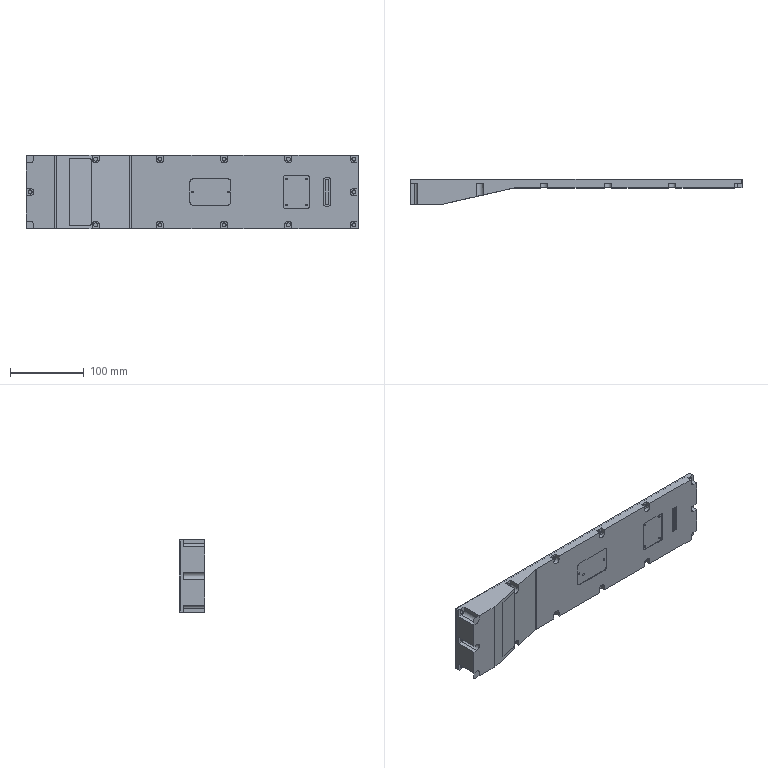NC program | Mastercam | posted with a generic post | part box 450 x 35 x 100 mm
Lines 24995 to 25762 of 140701:
(20 FEM |TOOL - 20|DIA. OFF. - 20|LEN. - 20|TOOL DIA. - 20.)
N556 T20 M6
N558 G0 G54 G90 X-118.202 Y-6.075 C0. B0. S7000 M3
N560 G43 H20 Z50.
N562 Z1.055
N564 G2 X-116.202 Y-4.075 Z1. I2. F4000.
N566 G3 X-97.202 Y14.925 Z.5 J19.
N568 X-116.202 Y33.925 Z0. I-19.
N570 X-135.202 Y14.925 Z-.5 J-19.
N572 X-116.202 Y-4.075 Z-1. I19.
N574 G1 X-91.853
N576 X-63.511
N578 G2 X-59.795 Y0. I43.131 J-35.6
N580 X-63.511 Y4.075 I39.415 J39.675
N582 G1 X-122.39
N584 Y-4.075
N586 X-116.202
N588 G2 X-114.191 Y-5.683 J-2.062
N590 G1 X-112.027 Y-15.257
N592 G3 X-110.015 Y-16.865 I2.012 J.455
N594 G1 X-91.853
N596 X-56.995
N598 G2 X-49.546 Y-7.894 I79.55 J-58.48
N600 X-41.146 Y-1.835 I29.252 J-31.701
N602 G1 X-37.436 Y0.
N604 X-41.146 Y1.835
N606 G2 X-49.546 Y7.894 I20.852 J37.76
N608 X-56.995 Y16.865 I72.101 J67.451
N610 G1 X-135.18
N612 Y-16.865
N614 X-110.015
N616 G3 X-108.015 Y-14.865 Z-.945 J2.
N618 G0 Z50.
N620 X42.897 Y-2.91
N622 Z1.
N624 G3 X51.894 Y-5.175 Z.843 I8.997 J16.735
N626 X68.629 Y4.827 Z.5 J19.
N628 X70.895 Y13.825 Z.343 I-16.735 J8.998
N630 X60.892 Y30.559 Z0. I-19.001
N632 X51.894 Y32.825 Z-.157 I-8.998 J-16.734
N634 X35.16 Y22.822 Z-.5 J-19.
N636 X32.895 Y13.825 Z-.657 I16.734 J-8.997
N638 X42.897 Y-2.91 Z-1. I18.999
N640 G2 X43.5 Y-3.234 I-391.044 J-727.301
N642 X49.572 Y0. I23.249 J-36.334
N644 X43.5 Y3.234 I17.177 J39.568
N646 X37.436 Y0. I-391.647 J726.977
N648 X42.897 Y-2.91 I-385.583 J-730.211
N650 G3 X43.844 Y-3.148 Z-.983 I.947 J1.762
N652 X45.605 Y-2.095 Z-.945 J2.
N654 G0 Z50.
N656 X129.904 Y-2.873
N658 Z1.
N660 G3 X139.687 Y-5.585 Z.828 I9.783 J16.288
N662 X155.975 Y3.632 Z.5 J19.
N664 X158.687 Y13.415 Z.328 I-16.288 J9.783
N666 X149.469 Y29.703 Z0. I-19.
N668 X139.687 Y32.415 Z-.172 I-9.782 J-16.288
N670 X123.399 Y23.197 Z-.5 J-19.
N672 X120.687 Y13.415 Z-.672 I16.288 J-9.782
N674 X129.904 Y-2.873 Z-1. I19.
N676 G2 X130.501 Y-3.237 I-27.641 J-46.024
N678 X136.397 Y-.078 I23.255 J-36.326
N680 G1 X136.575 Y0.
N682 X136.397 Y.078
N684 G2 X130.501 Y3.237 I17.359 J39.485
N686 X124.428 Y0. I-28.238 J45.66
N688 X129.904 Y-2.873 I-22.165 J-48.897
N690 X130.904 Y-4.641 I-1.062 J-1.768
N692 X130.837 Y-5.167 I-2.062
N694 G1 X128.644 Y-13.481
N696 G3 X128.576 Y-14.007 I1.995 J-.526
N698 X129.288 Y-15.566 I2.063
N700 G1 X130.501 Y-16.616
N702 G2 X135.006 Y-12.831 I23.174 J-23.004
N704 G1 X135.087 Y-12.774
N706 G2 X140.615 Y-9.672 I18.669 J-26.789
N708 G1 X140.702 Y-9.634
N710 G2 X146.548 Y-7.698 I13.141 J-29.891
N712 G1 X146.639 Y-7.677
N714 G2 X153.208 Y-6.86 I7.296 J-31.827
N716 G1 X153.401 Y-6.855
N718 X193.897 Y-6.847
N720 G2 X202.347 Y-7.916 I-1.055 J-42.291
N722 G1 Y7.916
N724 G2 X194.995 Y6.866 I-9.346 J39.174
N726 G1 X154.128 Y6.847
N728 X153.208 Y6.86
N730 G2 X146.639 Y7.677 I.727 J32.644
N732 G1 X146.548 Y7.698
N734 G2 X140.702 Y9.634 I7.295 J31.827
N736 G1 X140.615 Y9.672
N738 G2 X135.087 Y12.774 I13.141 J29.891
N740 G1 X135.006 Y12.831
N742 G2 X130.501 Y16.616 I18.669 J26.789
N744 G1 X126.823 Y13.429
N746 G2 X121.297 Y10.091 I-19.566 J26.142
N748 G1 X121.211 Y10.05
N750 G2 X109.473 Y6.942 I-14.658 J31.635
N752 G1 X109.381 Y6.935
N754 X67.041 Y6.847
N756 X66.081 Y6.861
N758 X60.698 Y7.454
N760 G2 X54.022 Y9.497 I6.163 J32.066
N762 G1 X53.91 Y9.545
N764 G2 X47.444 Y13.233 I12.839 J30.023
N766 G1 X43.499 Y16.616
N768 G2 X35.971 Y10.952 I-44.52 J51.336
N770 X25.649 Y7.333 I-16.878 J31.613
N772 G1 X20.337 Y6.85
N774 G2 X.051 Y6.761 I-20.286 J2311.595
N776 X-20.508 Y6.853 J2311.684
N778 X-30.199 Y8.456 I1.227 J37.504
N780 G1 X-30.263 Y8.477
N782 G2 X-35.971 Y10.952 I10.077 J31.059
N784 G1 X-36.079 Y11.012
N786 G2 X-42.437 Y15.598 I15.785 J28.583
N788 G1 X-42.523 Y15.677
N790 G2 X-47.502 Y21.493 I22.143 J23.998
N792 G1 X-47.568 Y21.591
N794 G2 X-50.642 Y27.347 I27.123 J18.181
N796 G1 X-145.662
N798 Y-27.347
N800 X-50.642
N802 G2 X-47.568 Y-21.591 I30.197 J-12.425
N804 G1 X-47.502 Y-21.493
N806 G2 X-42.523 Y-15.677 I27.122 J-18.182
N808 G1 X-42.437 Y-15.598
N810 G2 X-36.079 Y-11.012 I22.143 J-23.997
N812 G1 X-35.971 Y-10.952
N814 G2 X-30.263 Y-8.477 I15.785 J-28.584
N816 G1 X-30.199 Y-8.456
N818 G2 X-20.508 Y-6.853 I10.918 J-35.901
N820 X.051 Y-6.762 I20.559 J-2311.592
N822 X20.337 Y-6.85 J-2311.683
N824 G1 X25.649 Y-7.333
N826 G2 X35.971 Y-10.952 I-6.556 J-35.232
N828 X43.499 Y-16.616 I-36.992 J-57.
N830 G1 X47.444 Y-13.233
N832 G2 X53.91 Y-9.545 I19.305 J-26.335
N834 G1 X54.022 Y-9.497
N836 G2 X60.698 Y-7.454 I12.839 J-30.023
N838 G1 X60.788 Y-7.437
N840 G2 X67.041 Y-6.847 I6.861 J-39.333
N842 G1 X109.381 Y-6.935
N844 G2 X121.211 Y-10.05 I-2.812 J-34.699
N846 G1 X121.297 Y-10.091
N848 G2 X126.823 Y-13.429 I-14.04 J-29.48
N850 G1 X129.288 Y-15.566
N852 G2 X129.999 Y-17.124 I-1.351 J-1.558
N854 X129.767 Y-18.076 I-2.062
N856 G1 X124.991 Y-27.255
N858 G3 X124.758 Y-28.207 I1.83 J-.952
N860 X125.048 Y-29.262 I2.063
N862 G2 X128. Y-39.493 I-18.064 J-10.752
N864 G1 X133.001
N866 G2 X145.59 Y-20.752 I21.022 J-.523
N868 X153.478 Y-19.002 I8.921 J-21.56
N870 G1 X153.672 Y-18.998
N872 X193.897 Y-18.993
N874 X193.982
N876 G2 X214.493 Y-35.389 J-21.027
N878 G1 Y35.389
N880 G2 X194.768 Y19.011 I-20.505 J4.628
N882 G1 X194.587 Y19.005
N884 X153.672 Y18.998
N886 X149.261 Y19.537
N888 G2 X133.001 Y39.493 I4.758 J20.478
N890 G1 X128.
N892 G2 X112.383 Y19.696 I-21.016 J.521
N894 X106.99 Y18.993 I-13.4 J81.701
N896 G1 X66.495 Y19.
N898 G2 X54.539 Y23.091 I.65 J21.417
N900 X45.999 Y39.493 I12.534 J16.951
N902 G1 X41.
N904 G2 X39.774 Y32.921 I-49.58 J5.846
N906 G1 X39.731 Y32.803
N908 G2 X37.479 Y28.354 I-19.286 J6.969
N910 G1 X37.414 Y28.256
N912 G2 X34.287 Y24.604 I-17.034 J11.419
N914 G1 X34.201 Y24.524
N916 G2 X26.515 Y20.03 I-15.057 J16.929
N918 X20.337 Y18.997 I-7.888 J28.2
N920 X-.041 Y18.899 I-20.378 J2122.333
N922 X-20.166 Y18.995 J2122.431
N924 X-26.515 Y20.03 I1.337 J28.195
N926 X-34.287 Y24.604 I7.334 J21.352
N928 X-37.414 Y28.256 I13.907 J15.071
N930 G1 X-37.479 Y28.354
N932 G2 X-39.731 Y32.803 I17.034 J11.418
N934 X-41. Y39.493 I45.456 J12.083
N936 G1 X-157.808
N938 Y-39.493
N940 X-41.
N942 G2 X-39.774 Y-32.921 I49.58 J-5.846
N944 G1 X-39.731 Y-32.803
N946 G2 X-37.479 Y-28.354 I19.286 J-6.969
N948 G1 X-37.414 Y-28.256
N950 G2 X-34.287 Y-24.604 I17.034 J-11.419
N952 G1 X-34.201 Y-24.524
N954 G2 X-26.515 Y-20.03 I15.057 J-16.929
N956 X-20.337 Y-18.997 I7.888 J-28.2
N958 X.004 Y-18.899 I20.341 J-2118.094
N960 X19.878 Y-18.993 J-2118.192
N962 X26.515 Y-20.03 I-.812 J-26.956
N964 X34.201 Y-24.524 I-7.371 J-21.423
N966 G1 X34.287 Y-24.604
N968 G2 X37.414 Y-28.256 I-13.907 J-15.071
N970 G1 X37.479 Y-28.354
N972 G2 X39.731 Y-32.803 I-17.034 J-11.418
N974 X41. Y-39.493 I-45.456 J-12.083
N976 G1 X45.999
N978 G2 X51.434 Y-25.897 I21.203 J-.591
N980 X67.041 Y-18.993 I15.623 J-14.225
N982 G1 X106.99
N984 G2 X112.383 Y-19.696 I-8.007 J-82.404
N986 X125.048 Y-29.262 I-5.399 J-20.318
N988 X125.338 Y-30.316 I-1.772 J-1.054
N990 X124.805 Y-31.701 I-2.062
N992 G1 X118.034 Y-39.175
N994 G3 X117.5 Y-40.559 I1.528 J-1.385
N996 G1 X117.499 Y-50.
N998 X143.501
N1000 G2 X143.5 Y-49.884 I9.999 J.116
N1002 G1 X143.505 Y-39.753
N1004 X143.509 Y-39.626
N1006 G2 X143.82 Y-37.443 I9.995 J-.311
N1008 G1 X143.851 Y-37.322
N1010 G2 X144.5 Y-35.531 I9.684 J-2.493
N1012 G1 X144.527 Y-35.473
N1014 G2 X145.171 Y-34.319 I9.036 J-4.284
N1016 G1 X145.208 Y-34.262
N1018 G2 X146.3 Y-32.865 I8.392 J-5.438
N1020 G1 X146.375 Y-32.785
N1022 G2 X147.957 Y-31.416 I7.3 J-6.835
N1024 G1 X148.039 Y-31.359
N1026 G2 X149.732 Y-30.409 I5.717 J-8.204
N1028 G1 X149.818 Y-30.371
N1030 G2 X151.609 Y-29.778 I4.025 J-9.154
N1032 G1 X151.7 Y-29.757
N1034 G2 X153.712 Y-29.507 I2.235 J-9.747
N1036 G1 X153.905 Y-29.502
N1038 X193.897 Y-29.5
N1040 X194.414 Y-29.512
N1042 G2 X196.337 Y-29.765 I-.336 J-9.994
N1044 G1 X196.406 Y-29.781
N1046 G2 X197.7 Y-30.175 I-2.258 J-9.741
N1048 G1 X197.76 Y-30.197
N1050 G2 X199.353 Y-30.971 I-3.553 J-9.348
N1052 G1 X199.45 Y-31.029
N1054 G2 X201.184 Y-32.346 I-5.146 J-8.574
N1056 G1 X201.26 Y-32.418
N1058 G2 X202.596 Y-33.975 I-6.88 J-7.257
N1060 G1 X202.654 Y-34.058
N1062 G2 X203.635 Y-35.832 I-8.217 J-5.7
N1064 G1 X203.675 Y-35.926
N1066 G2 X204.291 Y-37.927 I-9.198 J-3.926
N1068 G1 X204.311 Y-38.033
N1070 G2 X204.497 Y-39.8 I-9.813 J-1.924
N1072 G1 X204.499 Y-39.917
N1074 Y-50.
N1076 X223.648
N1078 X223.993 Y-49.994
N1080 X224.033 Y-49.965
N1082 X224.98 Y-49.016
N1084 X224.995 Y-48.986
N1086 X225. Y-48.71
N1088 Y48.71
N1090 X224.995 Y48.986
N1092 X224.98 Y49.016
N1094 X224.033 Y49.965
N1096 X223.971 Y49.996
N1098 X204.499 Y50.
N1100 X204.5 Y40.074
N1102 X204.497 Y39.8
N1104 G2 X204.311 Y38.033 I-9.999 J.157
N1106 G1 X204.291 Y37.927
N1108 G2 X203.675 Y35.926 I-9.814 J1.925
N1110 G1 X203.635 Y35.832
N1112 G2 X202.654 Y34.058 I-9.198 J3.926
N1114 G1 X202.596 Y33.975
N1116 G2 X201.26 Y32.418 I-8.216 J5.7
N1118 G1 X201.184 Y32.346
N1120 G2 X199.45 Y31.029 I-6.88 J7.257
N1122 G1 X199.353 Y30.971
N1124 G2 X197.76 Y30.197 I-5.146 J8.574
N1126 G1 X197.7 Y30.175
N1128 G2 X196.406 Y29.781 I-3.552 J9.347
N1130 G1 X196.337 Y29.765
N1132 G2 X194.414 Y29.512 I-2.259 J9.741
N1134 G1 X193.897 Y29.5
N1136 X154.128
N1138 X153.712 Y29.507
N1140 G2 X151.7 Y29.757 I.223 J9.997
N1142 G1 X151.609 Y29.778
N1144 G2 X149.818 Y30.371 I2.234 J9.747
N1146 G1 X149.732 Y30.409
N1148 G2 X148.039 Y31.359 I4.024 J9.154
N1150 G1 X147.957 Y31.416
N1152 G2 X146.375 Y32.785 I5.718 J8.204
N1154 G1 X146.3 Y32.865
N1156 G2 X145.208 Y34.262 I7.3 J6.835
N1158 G1 X145.171 Y34.319
N1160 G2 X144.527 Y35.473 I8.392 J5.438
N1162 G1 X144.5 Y35.531
N1164 G2 X143.851 Y37.322 I9.035 J4.284
N1166 G1 X143.82 Y37.443
N1168 G2 X143.509 Y39.626 I9.684 J2.494
N1170 G1 X143.505 Y39.753
N1172 X143.501 Y50.
N1174 X117.499
N1176 X117.5 Y40.041
N1178 X117.458 Y39.11
N1180 G2 X117.074 Y37.042 I-9.97 J.783
N1182 G1 X117.053 Y36.973
N1184 G2 X116.533 Y35.602 I-9.585 J2.85
N1186 G1 X116.502 Y35.535
N1188 G2 X115.768 Y34.226 I-9.066 J4.221
N1190 G1 X115.726 Y34.162
N1192 G2 X114.752 Y32.92 I-8.332 J5.53
N1194 G1 X114.697 Y32.86
N1196 G2 X113.331 Y31.627 I-7.358 J6.773
N1198 G1 X113.249 Y31.565
N1200 G2 X111.557 Y30.543 I-5.992 J8.006
N1202 G1 X111.471 Y30.502
N1204 G2 X109.712 Y29.858 I-4.3 J9.028
N1206 G1 X109.623 Y29.835
N1208 G2 X107.814 Y29.534 I-2.541 J9.672
N1210 G1 X106.99 Y29.5
N1212 X67.041
N1214 X66.685 Y29.506
N1216 G2 X65.063 Y29.682 I.266 J9.996
N1218 G1 X64.974 Y29.699
N1220 G2 X62.929 Y30.325 I1.887 J9.821
N1222 G1 X62.817 Y30.373
N1224 G2 X60.837 Y31.503 I3.932 J9.195
N1226 G1 X60.751 Y31.565
N1228 G2 X59.237 Y32.933 I5.912 J8.065
N1230 G1 X59.171 Y33.006
N1232 G2 X58.019 Y34.565 I7.427 J6.697
N1234 G1 X57.97 Y34.647
N1236 G2 X57.146 Y36.381 I8.578 J5.138
N1238 G1 X57.113 Y36.472
N1240 G2 X56.627 Y38.39 I9.403 J3.404
N1242 G1 X56.612 Y38.49
N1244 G2 X56.501 Y39.95 I9.889 J1.486
N1246 G1 X56.5 Y40.166
N1248 X56.501 Y50.
N1250 X30.499
N1252 X30.5 Y40.036
N1254 X30.453 Y39.059
N1256 G2 X29.893 Y36.492 I-9.965 J.831
N1258 G1 X29.85 Y36.374
N1260 G2 X28.752 Y34.204 I-9.405 J3.398
N1262 G1 X28.686 Y34.107
N1264 G2 X27.161 Y32.325 I-8.306 J5.568
N1266 G1 X27.075 Y32.246
N1268 G2 X25.128 Y30.842 I-6.781 J7.349
N1270 G1 X25.02 Y30.782
N1272 G2 X23.272 Y30.024 I-4.834 J8.754
N1274 G1 X23.208 Y30.003
N1276 G2 X21.837 Y29.663 I-3.086 J9.512
N1278 G1 X21.764 Y29.651
N1280 G2 X20.19 Y29.503 I-1.715 J9.851
N1282 G1 X19.878 Y29.5
N1284 X-20.018 Y29.501
N1286 X-20.19 Y29.503
N1288 G2 X-21.764 Y29.651 I.141 J9.999
N1290 G1 X-21.837 Y29.663
N1292 G2 X-23.208 Y30.003 I1.715 J9.852
N1294 G1 X-23.272 Y30.024
N1296 G2 X-25.02 Y30.782 I3.086 J9.512
N1298 G1 X-25.128 Y30.842
N1300 G2 X-27.075 Y32.246 I4.834 J8.753
N1302 G1 X-27.161 Y32.325
N1304 G2 X-28.686 Y34.107 I6.781 J7.35
N1306 G1 X-28.752 Y34.204
N1308 G2 X-29.85 Y36.374 I8.307 J5.568
N1310 G1 X-29.893 Y36.492
N1312 G2 X-30.453 Y39.059 I9.405 J3.398
N1314 G1 X-30.5 Y40.036
N1316 X-30.499 Y50.
N1318 X-168.315
N1320 Y-50.
N1322 X-30.499
N1324 X-30.5 Y-40.036
N1326 X-30.453 Y-39.059
N1328 G2 X-29.893 Y-36.492 I9.965 J-.831
N1330 G1 X-29.85 Y-36.374
N1332 G2 X-28.752 Y-34.204 I9.405 J-3.398
N1334 G1 X-28.686 Y-34.107
N1336 G2 X-27.161 Y-32.325 I8.306 J-5.568
N1338 G1 X-27.075 Y-32.246
N1340 G2 X-25.128 Y-30.842 I6.781 J-7.349
N1342 G1 X-25.02 Y-30.782
N1344 G2 X-23.272 Y-30.024 I4.834 J-8.754
N1346 G1 X-23.208 Y-30.003
N1348 G2 X-21.837 Y-29.663 I3.086 J-9.512
N1350 G1 X-21.764 Y-29.651
N1352 G2 X-20.19 Y-29.503 I1.715 J-9.851
N1354 G1 X-19.878 Y-29.5
N1356 X20.018 Y-29.501
N1358 X20.19 Y-29.503
N1360 G2 X21.764 Y-29.651 I-.141 J-9.999
N1362 G1 X21.837 Y-29.663
N1364 G2 X23.208 Y-30.003 I-1.715 J-9.852
N1366 G1 X23.272 Y-30.024
N1368 G2 X25.02 Y-30.782 I-3.086 J-9.512
N1370 G1 X25.128 Y-30.842
N1372 G2 X27.075 Y-32.246 I-4.834 J-8.753
N1374 G1 X27.161 Y-32.325
N1376 G2 X28.686 Y-34.107 I-6.781 J-7.35
N1378 G1 X28.752 Y-34.204
N1380 G2 X29.85 Y-36.374 I-8.307 J-5.568
N1382 G1 X29.893 Y-36.492
N1384 G2 X30.453 Y-39.059 I-9.405 J-3.398
N1386 G1 X30.5 Y-40.036
N1388 X30.499 Y-50.
N1390 X56.501
N1392 Y-39.976
N1394 G2 X56.612 Y-38.49 I10.
N1396 G1 X56.627 Y-38.39
N1398 G2 X57.113 Y-36.472 I9.889 J-1.486
N1400 G1 X57.146 Y-36.381
N1402 G2 X57.97 Y-34.647 I9.402 J-3.404
N1404 G1 X58.019 Y-34.565
N1406 G2 X59.171 Y-33.006 I8.579 J-5.138
N1408 G1 X59.237 Y-32.933
N1410 G2 X60.751 Y-31.565 I7.426 J-6.697
N1412 G1 X60.837 Y-31.503
N1414 G2 X62.817 Y-30.373 I5.912 J-8.065
N1416 G1 X62.929 Y-30.325
N1418 G2 X64.974 Y-29.699 I3.932 J-9.195
N1420 G1 X65.063 Y-29.682
N1422 G2 X66.685 Y-29.506 I1.888 J-9.82
N1424 G1 X67.041 Y-29.5
N1426 X106.99
N1428 X107.814 Y-29.534
N1430 G2 X109.623 Y-29.835 I-.732 J-9.973
N1432 G1 X109.712 Y-29.858
N1434 G2 X111.471 Y-30.502 I-2.541 J-9.672
N1436 G1 X111.557 Y-30.543
N1438 G2 X113.249 Y-31.565 I-4.3 J-9.028
N1440 G1 X113.331 Y-31.627
N1442 G2 X114.697 Y-32.86 I-5.992 J-8.006
N1444 G1 X114.752 Y-32.92
N1446 G2 X115.726 Y-34.162 I-7.358 J-6.772
N1448 G1 X115.768 Y-34.226
N1450 G2 X116.502 Y-35.535 I-8.332 J-5.53
N1452 G1 X116.533 Y-35.602
N1454 G2 X117.053 Y-36.973 I-9.065 J-4.221
N1456 G1 X117.074 Y-37.042
N1458 G2 X117.458 Y-39.11 I-9.586 J-2.851
N1460 G1 X117.469 Y-39.258
N1462 G2 X117.5 Y-40.041 I-9.969 J-.783
N1464 G1 Y-40.559
N1466 Y-40.56
N1468 G3 X119.562 Y-42.622 I2.062
N1470 X121.427 Y-41.442 J2.062
N1472 G1 X145.254 Y8.886
N1474 G3 X147.082 Y17.017 Z-1.079 I-17.172 J8.131
N1476 X130.973 Y35.795 Z-1.333 I-19.
N1478 X128.082 Y36.016 Z-1.36 I-2.891 J-18.778
N1480 X109.083 Y17.017 Z-1.642 J-18.999
N1482 X109.259 Y14.429 Z-1.667 I18.999
N1484 X128.082 Y-1.983 Z-1.924 I18.823 J2.588
N1486 X135.933 Y-.285 Z-2. J19.
N1488 G2 X136.397 Y-.078 I17.823 J-39.278
N1490 G1 X136.575 Y0.
N1492 X136.397 Y.078
N1494 G2 X130.501 Y3.237 I17.359 J39.485
N1496 X124.428 Y0. I-28.238 J45.66
N1498 X130.501 Y-3.237 I-22.165 J-48.897
N1500 X135.933 Y-.285 I23.255 J-36.326
N1502 G3 X137.106 Y1.536 Z-1.96 I-.827 J1.821
N1504 X136.928 Y2.362 Z-1.945 I-2.
N1506 G0 Z50.
N1508 X44.092 Y2.862
N1510 Z0.
N1512 G3 X34.112 Y5.694 Z-.176 I-9.98 J-16.168
N1514 X17.944 Y-3.327 Z-.5 J-19.
N1516 X15.112 Y-13.306 Z-.676 I16.168 J-9.979
N1518 X24.133 Y-29.474 Z-1. I19.
N1520 X34.112 Y-32.306 Z-1.176 I9.979 J16.168
N1522 X50.28 Y-23.286 Z-1.5 J19.
N1524 X53.112 Y-13.306 Z-1.676 I-16.168 J9.98
N1526 X44.092 Y2.862 Z-2. I-19.
N1528 G2 X43.5 Y3.234 I22.657 J36.706
N1530 X37.436 Y0. I-391.647 J726.977
N1532 X43.5 Y-3.234 I-385.583 J-730.211
N1534 X49.572 Y0. I23.249 J-36.334
N1536 X44.092 Y2.862 I17.177 J39.568
N1538 G3 X43.042 Y3.16 Z-1.981 I-1.05 J-1.702
N1540 X41.34 Y2.21 Z-1.945 J-2.
N1542 G0 Z50.
N1544 X-64.181 Y4.075
N1546 Z0.
N1548 G3 X-83.181 Y-14.925 Z-.5 J-19.
N1550 X-64.181 Y-33.925 Z-1. I19.
N1552 X-45.181 Y-14.925 Z-1.5 J19.
N1554 X-64.181 Y4.075 Z-2. I-19.
N1556 G1 X-117.97
N1558 Y-4.075
N1560 X-89.643
N1562 X-63.511
N1564 G2 X-59.795 Y0. I43.131 J-35.6
N1566 X-63.511 Y4.075 I39.415 J39.675
N1568 G1 X-64.181
N1570 G2 X-66.193 Y5.683 J2.062
N1572 G1 X-68.357 Y15.257
N1574 G3 X-70.369 Y16.865 I-2.012 J-.455
N1576 G1 X-130.761
N1578 Y-16.865
N1580 X-89.643
N1582 X-56.995
N1584 G2 X-49.546 Y-7.894 I79.55 J-58.48
N1586 X-41.146 Y-1.835 I29.252 J-31.701
N1588 G1 X-37.436 Y0.
N1590 X-41.146 Y1.835
N1592 G2 X-49.546 Y7.894 I20.852 J37.76
N1594 X-56.995 Y16.865 I72.101 J67.451
N1596 G1 X-70.369
N1598 G2 X-72.346 Y18.341 J2.062
N1600 G1 X-74.579 Y25.871
N1602 G3 X-76.556 Y27.347 I-1.977 J-.586
N1604 G1 X-141.243
N1606 Y-27.347
N1608 X-50.642
N1610 G2 X-47.568 Y-21.591 I30.197 J-12.425
N1612 G1 X-47.502 Y-21.493
N1614 G2 X-42.523 Y-15.677 I27.122 J-18.182
N1616 G1 X-42.437 Y-15.598
N1618 G2 X-36.079 Y-11.012 I22.143 J-23.997
N1620 G1 X-35.971 Y-10.952
N1622 G2 X-30.263 Y-8.477 I15.785 J-28.584
N1624 G1 X-30.199 Y-8.456
N1626 G2 X-20.508 Y-6.853 I10.918 J-35.901
N1628 X.051 Y-6.762 I20.559 J-2311.592
N1630 X20.337 Y-6.85 J-2311.683
N1632 G1 X25.649 Y-7.333
N1634 G2 X35.971 Y-10.952 I-6.556 J-35.232
N1636 X43.499 Y-16.616 I-36.992 J-57.
N1638 G1 X47.444 Y-13.233
N1640 G2 X53.91 Y-9.545 I19.305 J-26.335
N1642 G1 X54.022 Y-9.497
N1644 G2 X60.698 Y-7.454 I12.839 J-30.023
N1646 G1 X60.788 Y-7.437
N1648 G2 X67.041 Y-6.847 I6.861 J-39.333
N1650 G1 X109.381 Y-6.935
N1652 G2 X121.211 Y-10.05 I-2.812 J-34.699
N1654 G1 X121.297 Y-10.091
N1656 G2 X126.823 Y-13.429 I-14.04 J-29.48
N1658 G1 X130.501 Y-16.616
N1660 G2 X135.006 Y-12.831 I23.174 J-23.004
N1662 G1 X135.087 Y-12.774
N1664 G2 X140.615 Y-9.672 I18.669 J-26.789
N1666 G1 X140.702 Y-9.634
N1668 G2 X146.548 Y-7.698 I13.141 J-29.891
N1670 G1 X146.639 Y-7.677
N1672 G2 X153.208 Y-6.86 I7.296 J-31.827
N1674 G1 X153.401 Y-6.855
N1676 X193.897 Y-6.847
N1678 G2 X202.347 Y-7.916 I-1.055 J-42.291
N1680 G1 Y7.916
N1682 G2 X194.995 Y6.866 I-9.346 J39.174
N1684 G1 X154.128 Y6.847
N1686 X153.208 Y6.86
N1688 G2 X146.639 Y7.677 I.727 J32.644
N1690 G1 X146.548 Y7.698
N1692 G2 X140.702 Y9.634 I7.295 J31.827
N1694 G1 X140.615 Y9.672
N1696 G2 X135.087 Y12.774 I13.141 J29.891
N1698 G1 X135.006 Y12.831
N1700 G2 X130.501 Y16.616 I18.669 J26.789
N1702 G1 X126.823 Y13.429
N1704 G2 X121.297 Y10.091 I-19.566 J26.142
N1706 G1 X121.211 Y10.05
N1708 G2 X109.473 Y6.942 I-14.658 J31.635
N1710 G1 X109.381 Y6.935
N1712 X67.041 Y6.847
N1714 X66.081 Y6.861
N1716 X60.698 Y7.454
N1718 G2 X54.022 Y9.497 I6.163 J32.066
N1720 G1 X53.91 Y9.545
N1722 G2 X47.444 Y13.233 I12.839 J30.023
N1724 G1 X43.499 Y16.616
N1726 G2 X35.971 Y10.952 I-44.52 J51.336
N1728 X25.649 Y7.333 I-16.878 J31.613
N1730 G1 X20.337 Y6.85
N1732 G2 X.051 Y6.761 I-20.286 J2311.595
N1734 X-20.508 Y6.853 J2311.684
N1736 X-30.199 Y8.456 I1.227 J37.504
N1738 G1 X-30.263 Y8.477
N1740 G2 X-35.971 Y10.952 I10.077 J31.059
N1742 G1 X-36.079 Y11.012
N1744 G2 X-42.437 Y15.598 I15.785 J28.583
N1746 G1 X-42.523 Y15.677
N1748 G2 X-47.502 Y21.493 I22.143 J23.998
N1750 G1 X-47.568 Y21.591
N1752 G2 X-50.642 Y27.347 I27.123 J18.181
N1754 G1 X-76.556
N1756 G2 X-78.561 Y28.924 J2.063
N1758 G1 X-80.739 Y37.916
N1760 G3 X-82.744 Y39.493 I-2.005 J-.486
N1762 G1 X-153.389
N1764 Y-39.493
N1766 X-41.
N1768 G2 X-39.774 Y-32.921 I49.58 J-5.846
N1770 G1 X-39.731 Y-32.803
N1772 G2 X-37.479 Y-28.354 I19.286 J-6.969
N1774 G1 X-37.414 Y-28.256
N1776 G2 X-34.287 Y-24.604 I17.034 J-11.419
N1778 G1 X-34.201 Y-24.524
N1780 G2 X-26.515 Y-20.03 I15.057 J-16.929
N1782 X-20.337 Y-18.997 I7.888 J-28.2
N1784 X.004 Y-18.899 I20.341 J-2118.094
N1786 X19.878 Y-18.993 J-2118.192
N1788 X26.515 Y-20.03 I-.812 J-26.956
N1790 X34.201 Y-24.524 I-7.371 J-21.423
N1792 G1 X34.287 Y-24.604
N1794 G2 X37.414 Y-28.256 I-13.907 J-15.071
N1796 G1 X37.479 Y-28.354
N1798 G2 X39.731 Y-32.803 I-17.034 J-11.418
N1800 X41. Y-39.493 I-45.456 J-12.083
N1802 G1 X45.999
N1804 G2 X51.434 Y-25.897 I21.203 J-.591
N1806 X67.041 Y-18.993 I15.623 J-14.225
N1808 G1 X106.99
N1810 G2 X112.383 Y-19.696 I-8.007 J-82.404
N1812 X128. Y-39.493 I-5.399 J-20.318
N1814 G1 X133.001
N1816 G2 X145.59 Y-20.752 I21.022 J-.523
N1818 X153.478 Y-19.002 I8.921 J-21.56
N1820 G1 X153.672 Y-18.998
N1822 X193.897 Y-18.993
N1824 X193.982
N1826 G2 X214.493 Y-35.389 J-21.027
N1828 G1 Y35.389
N1830 G2 X194.768 Y19.011 I-20.505 J4.628
N1832 G1 X194.587 Y19.005
N1834 X153.672 Y18.998
N1836 X149.261 Y19.537
N1838 G2 X133.001 Y39.493 I4.758 J20.478
N1840 G1 X128.
N1842 G2 X112.383 Y19.696 I-21.016 J.521
N1844 X106.99 Y18.993 I-13.4 J81.701
N1846 G1 X66.495 Y19.
N1848 G2 X54.539 Y23.091 I.65 J21.417
N1850 X45.999 Y39.493 I12.534 J16.951
N1852 G1 X41.
N1854 G2 X39.774 Y32.921 I-49.58 J5.846
N1856 G1 X39.731 Y32.803
N1858 G2 X37.479 Y28.354 I-19.286 J6.969
N1860 G1 X37.414 Y28.256
N1862 G2 X34.287 Y24.604 I-17.034 J11.419
N1864 G1 X34.201 Y24.524
N1866 G2 X26.515 Y20.03 I-15.057 J16.929
N1868 X20.337 Y18.997 I-7.888 J28.2
N1870 X-.041 Y18.899 I-20.378 J2122.333
N1872 X-20.166 Y18.995 J2122.431
N1874 X-26.515 Y20.03 I1.337 J28.195
N1876 X-34.287 Y24.604 I7.334 J21.352
N1878 X-37.414 Y28.256 I13.907 J15.071
N1880 G1 X-37.479 Y28.354
N1882 G2 X-39.731 Y32.803 I17.034 J11.418
N1884 X-41. Y39.493 I45.456 J12.083
N1886 G1 X-82.744
N1888 G2 X-84.722 Y40.971 J2.062
N1890 G1 X-86.953 Y48.522
N1892 G3 X-88.931 Y50. I-1.978 J-.584
N1894 G1 X-163.896
N1896 Y-50.
N1898 X-30.499
N1900 X-30.5 Y-40.036
N1902 X-30.453 Y-39.059
N1904 G2 X-29.893 Y-36.492 I9.965 J-.831
N1906 G1 X-29.85 Y-36.374
N1908 G2 X-28.752 Y-34.204 I9.405 J-3.398
N1910 G1 X-28.686 Y-34.107
N1912 G2 X-27.161 Y-32.325 I8.306 J-5.568
N1914 G1 X-27.075 Y-32.246
N1916 G2 X-25.128 Y-30.842 I6.781 J-7.349
N1918 G1 X-25.02 Y-30.782
N1920 G2 X-23.272 Y-30.024 I4.834 J-8.754
N1922 G1 X-23.208 Y-30.003
N1924 G2 X-21.837 Y-29.663 I3.086 J-9.512
N1926 G1 X-21.764 Y-29.651
N1928 G2 X-20.19 Y-29.503 I1.715 J-9.851
N1930 G1 X-19.878 Y-29.5
N1932 X20.018 Y-29.501
N1934 X20.19 Y-29.503
N1936 G2 X21.764 Y-29.651 I-.141 J-9.999
N1938 G1 X21.837 Y-29.663
N1940 G2 X23.208 Y-30.003 I-1.715 J-9.852
N1942 G1 X23.272 Y-30.024
N1944 G2 X25.02 Y-30.782 I-3.086 J-9.512
N1946 G1 X25.128 Y-30.842
N1948 G2 X27.075 Y-32.246 I-4.834 J-8.753
N1950 G1 X27.161 Y-32.325
N1952 G2 X28.686 Y-34.107 I-6.781 J-7.35
N1954 G1 X28.752 Y-34.204
N1956 G2 X29.85 Y-36.374 I-8.307 J-5.568
N1958 G1 X29.893 Y-36.492
N1960 G2 X30.453 Y-39.059 I-9.405 J-3.398
N1962 G1 X30.5 Y-40.036
N1964 X30.499 Y-50.
N1966 X56.501
N1968 Y-39.976
N1970 G2 X56.612 Y-38.49 I10.
N1972 G1 X56.627 Y-38.39
N1974 G2 X57.113 Y-36.472 I9.889 J-1.486
N1976 G1 X57.146 Y-36.381
N1978 G2 X57.97 Y-34.647 I9.402 J-3.404
N1980 G1 X58.019 Y-34.565
N1982 G2 X59.171 Y-33.006 I8.579 J-5.138
N1984 G1 X59.237 Y-32.933
N1986 G2 X60.751 Y-31.565 I7.426 J-6.697
N1988 G1 X60.837 Y-31.503
N1990 G2 X62.817 Y-30.373 I5.912 J-8.065
N1992 G1 X62.929 Y-30.325
N1994 G2 X64.974 Y-29.699 I3.932 J-9.195
N1996 G1 X65.063 Y-29.682
N1998 G2 X66.685 Y-29.506 I1.888 J-9.82
N2000 G1 X67.041 Y-29.5
N2002 X106.99
N2004 X107.814 Y-29.534
N2006 G2 X109.623 Y-29.835 I-.732 J-9.973
N2008 G1 X109.712 Y-29.858
N2010 G2 X111.471 Y-30.502 I-2.541 J-9.672
N2012 G1 X111.557 Y-30.543
N2014 G2 X113.249 Y-31.565 I-4.3 J-9.028
N2016 G1 X113.331 Y-31.627
N2018 G2 X114.697 Y-32.86 I-5.992 J-8.006
N2020 G1 X114.752 Y-32.92
N2022 G2 X115.726 Y-34.162 I-7.358 J-6.772
N2024 G1 X115.768 Y-34.226
N2026 G2 X116.502 Y-35.535 I-8.332 J-5.53
N2028 G1 X116.533 Y-35.602
N2030 G2 X117.053 Y-36.973 I-9.065 J-4.221
N2032 G1 X117.074 Y-37.042
N2034 G2 X117.458 Y-39.11 I-9.586 J-2.851
N2036 G1 X117.469 Y-39.258
N2038 G2 X117.5 Y-40.041 I-9.969 J-.783
N2040 G1 X117.499 Y-50.
N2042 X143.501
N2044 G2 X143.5 Y-49.884 I9.999 J.116
N2046 G1 X143.505 Y-39.753
N2048 X143.509 Y-39.626
N2050 G2 X143.82 Y-37.443 I9.995 J-.311
N2052 G1 X143.851 Y-37.322
N2054 G2 X144.5 Y-35.531 I9.684 J-2.493
N2056 G1 X144.527 Y-35.473
N2058 G2 X145.171 Y-34.319 I9.036 J-4.284
N2060 G1 X145.208 Y-34.262
N2062 G2 X146.3 Y-32.865 I8.392 J-5.438
N2064 G1 X146.375 Y-32.785
N2066 G2 X147.957 Y-31.416 I7.3 J-6.835
N2068 G1 X148.039 Y-31.359
N2070 G2 X149.732 Y-30.409 I5.717 J-8.204
N2072 G1 X149.818 Y-30.371
N2074 G2 X151.609 Y-29.778 I4.025 J-9.154
N2076 G1 X151.7 Y-29.757
N2078 G2 X153.712 Y-29.507 I2.235 J-9.747
N2080 G1 X153.905 Y-29.502
N2082 X193.897 Y-29.5
N2084 X194.414 Y-29.512
N2086 G2 X196.337 Y-29.765 I-.336 J-9.994
N2088 G1 X196.406 Y-29.781